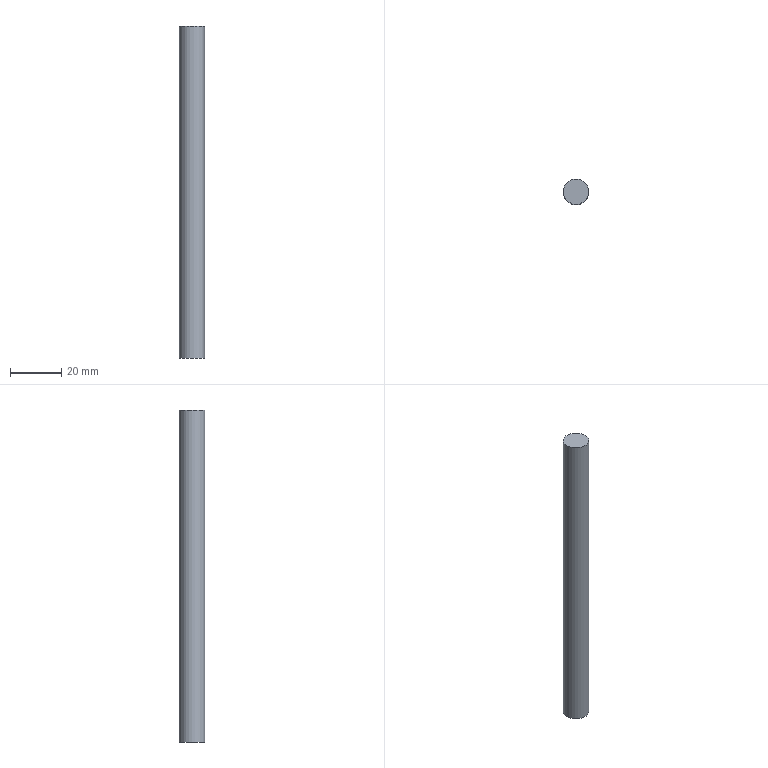Part | NX | features DATUM_CSYS 2, EXTRUDE 1, SKETCH 1 | 1 solid | 3 faces | box 10 x 10 x 130 mm | volume 10210 mm3 | plane 2 | cylinder 1 | commonest cylinder face diameters 10 x1
STEP:
#1=CARTESIAN_POINT('',(5.,0.,130.));
#2=VERTEX_POINT('',#1);
#3=CARTESIAN_POINT('',(0.,0.,130.));
#4=DIRECTION('',(0.,0.,1.));
#5=DIRECTION('',(1.,0.,0.));
#6=AXIS2_PLACEMENT_3D('',#3,#4,#5);
#7=CIRCLE('',#6,5.);
#8=EDGE_CURVE('',#2,#2,#7,.T.);
#9=ORIENTED_EDGE('',*,*,#8,.F.);
#10=EDGE_LOOP('',(#9));
#11=FACE_BOUND('',#10,.T.);
#12=CARTESIAN_POINT('',(5.,0.,0.));
#13=VERTEX_POINT('',#12);
#14=CARTESIAN_POINT('',(0.,0.,0.));
#15=DIRECTION('',(0.,0.,1.));
#16=DIRECTION('',(1.,0.,0.));
#17=AXIS2_PLACEMENT_3D('',#14,#15,#16);
#18=CIRCLE('',#17,5.);
#19=EDGE_CURVE('',#13,#13,#18,.T.);
#20=ORIENTED_EDGE('',*,*,#19,.T.);
#21=EDGE_LOOP('',(#20));
#22=FACE_BOUND('',#21,.T.);
#23=CARTESIAN_POINT('',(0.,0.,130.));
#24=DIRECTION('',(0.,0.,-1.));
#25=DIRECTION('',(-1.,0.,0.));
#26=AXIS2_PLACEMENT_3D('',#23,#24,#25);
#27=CYLINDRICAL_SURFACE('',#26,5.);
#28=ADVANCED_FACE('',(#11,#22),#27,.T.);
#29=ORIENTED_EDGE('',*,*,#8,.T.);
#30=EDGE_LOOP('',(#29));
#31=FACE_BOUND('',#30,.T.);
#32=CARTESIAN_POINT('',(0.,0.,130.));
#33=DIRECTION('',(0.,0.,1.));
#34=DIRECTION('',(1.,0.,0.));
#35=AXIS2_PLACEMENT_3D('',#32,#33,#34);
#36=PLANE('',#35);
#37=ADVANCED_FACE('',(#31),#36,.T.);
#38=ORIENTED_EDGE('',*,*,#19,.F.);
#39=EDGE_LOOP('',(#38));
#40=FACE_BOUND('',#39,.T.);
#41=CARTESIAN_POINT('',(0.,0.,0.));
#42=DIRECTION('',(0.,0.,1.));
#43=DIRECTION('',(1.,0.,0.));
#44=AXIS2_PLACEMENT_3D('',#41,#42,#43);
#45=PLANE('',#44);
#46=ADVANCED_FACE('',(#40),#45,.F.);
#47=CLOSED_SHELL('',(#28,#37,#46));
#48=MANIFOLD_SOLID_BREP('',#47);
#49=(LENGTH_UNIT()NAMED_UNIT(*)SI_UNIT(.MILLI.,.METRE.));
#50=UNCERTAINTY_MEASURE_WITH_UNIT(LENGTH_MEASURE(0.00001),#49,'','');
#51=(NAMED_UNIT(*)PLANE_ANGLE_UNIT()SI_UNIT($,.RADIAN.));
#52=(NAMED_UNIT(*)SI_UNIT($,.STERADIAN.)SOLID_ANGLE_UNIT());
#53=(GEOMETRIC_REPRESENTATION_CONTEXT(3)GLOBAL_UNCERTAINTY_ASSIGNED_CONTEXT((#50))GLOBAL_UNIT_ASSIGNED_CONTEXT((#49,#51,#52))REPRESENTATION_CONTEXT('',''));
#54=ADVANCED_BREP_SHAPE_REPRESENTATION('',(#48),#53);